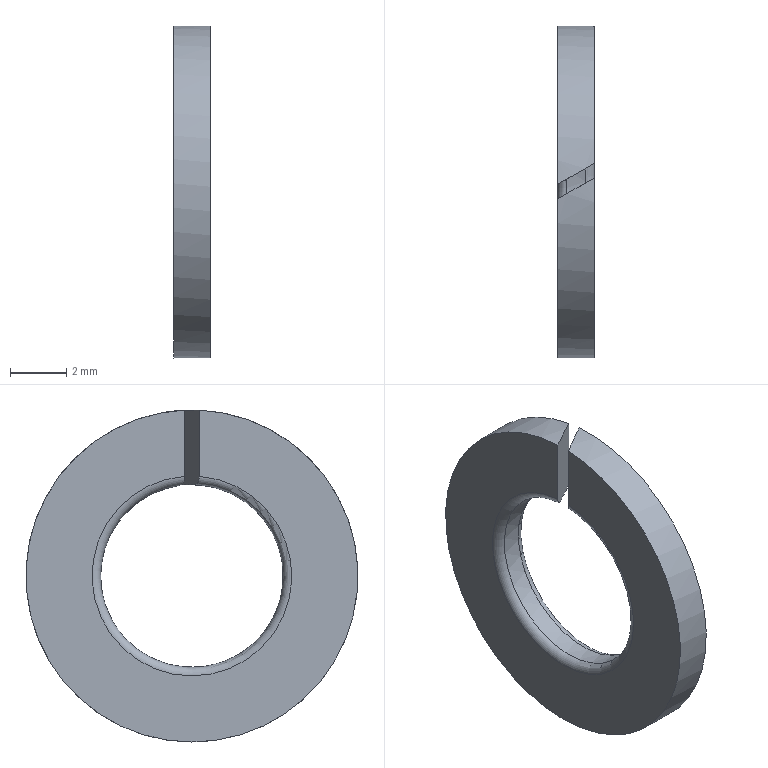Part | STEP file | DIN 128 - A6 | 1 solid | 8 faces | box 1.3 x 11.8 x 11.8 mm | volume 96.442 mm3 | plane 4 | cylinder 2 | torus 2 | commonest cylinder face diameters 6.5 x1 11.8 x1
STEP:
#1=CARTESIAN_POINT('',(0.,0.,0.));
#2=DIRECTION('',(0.,0.,1.));
#3=DIRECTION('',(1.,0.,0.));
#4=AXIS2_PLACEMENT_3D('',#1,#2,#3);
#5=CARTESIAN_POINT('',(1.3,1.011,3.403));
#6=VERTEX_POINT('',#5);
#7=CARTESIAN_POINT('',(1.,0.8374,3.14));
#8=VERTEX_POINT('',#7);
#9=CARTESIAN_POINT('',(1.3,1.011,3.403));
#10=CARTESIAN_POINT('',(1.3,1.011,3.366));
#11=CARTESIAN_POINT('',(1.292,1.006,3.323));
#12=CARTESIAN_POINT('',(1.265,0.9903,3.257));
#13=CARTESIAN_POINT('',(1.241,0.9768,3.224));
#14=CARTESIAN_POINT('',(1.191,0.9476,3.177));
#15=CARTESIAN_POINT('',(1.155,0.9267,3.157));
#16=CARTESIAN_POINT('',(1.085,0.8863,3.137));
#17=CARTESIAN_POINT('',(1.038,0.8595,3.134));
#18=CARTESIAN_POINT('',(1.,0.8374,3.14));
#19=B_SPLINE_CURVE_WITH_KNOTS('',3,(#9,#10,#11,#12,#13,#14,#15,#16,#17,#18),.UNSPECIFIED.,.F.,.F.,(4,2,2,2,4),(0.05089,0.06193,0.07271,0.08431,0.09772),.UNSPECIFIED.);
#20=CARTESIAN_POINT('',(0.,0.26,0.));
#21=DIRECTION('',(-0.5,0.866,0.));
#22=DIRECTION('',(0.,0.,1.));
#23=AXIS2_PLACEMENT_3D('',#20,#21,#22);
#24=PLANE('',#23);
#25=CARTESIAN_POINT('',(3.403,1.501));
#26=CARTESIAN_POINT('',(3.366,1.501));
#27=CARTESIAN_POINT('',(3.323,1.492));
#28=CARTESIAN_POINT('',(3.257,1.461));
#29=CARTESIAN_POINT('',(3.224,1.434));
#30=CARTESIAN_POINT('',(3.177,1.375));
#31=CARTESIAN_POINT('',(3.157,1.333));
#32=CARTESIAN_POINT('',(3.137,1.253));
#33=CARTESIAN_POINT('',(3.134,1.199));
#34=CARTESIAN_POINT('',(3.14,1.155));
#35=B_SPLINE_CURVE_WITH_KNOTS('',3,(#25,#26,#27,#28,#29,#30,#31,#32,#33,#34),.UNSPECIFIED.,.F.,.F.,(4,2,2,2,4),(0.05089,0.06193,0.07271,0.08431,0.09772),.UNSPECIFIED.);
#36=(GEOMETRIC_REPRESENTATION_CONTEXT(2)PARAMETRIC_REPRESENTATION_CONTEXT()REPRESENTATION_CONTEXT('',''));
#37=DEFINITIONAL_REPRESENTATION('',(#35),#36);
#38=PCURVE('',#24,#37);
#39=CARTESIAN_POINT('',(1.,0.,0.));
#40=DIRECTION('',(-1.,0.,0.));
#41=DIRECTION('',(0.,0.,1.));
#42=AXIS2_PLACEMENT_3D('',#39,#40,#41);
#43=TOROIDAL_SURFACE('',#42,3.55,0.3);
#44=CARTESIAN_POINT('',(0.2887,4.712));
#45=CARTESIAN_POINT('',(0.2892,4.69));
#46=CARTESIAN_POINT('',(0.2903,4.643));
#47=CARTESIAN_POINT('',(0.2918,4.568));
#48=CARTESIAN_POINT('',(0.293,4.492));
#49=CARTESIAN_POINT('',(0.2939,4.416));
#50=CARTESIAN_POINT('',(0.2945,4.343));
#51=CARTESIAN_POINT('',(0.2948,4.271));
#52=CARTESIAN_POINT('',(0.2947,4.195));
#53=CARTESIAN_POINT('',(0.2942,4.118));
#54=CARTESIAN_POINT('',(0.2935,4.041));
#55=CARTESIAN_POINT('',(0.2925,3.968));
#56=CARTESIAN_POINT('',(0.2911,3.899));
#57=CARTESIAN_POINT('',(0.2894,3.825));
#58=CARTESIAN_POINT('',(0.2874,3.751));
#59=CARTESIAN_POINT('',(0.2851,3.678));
#60=CARTESIAN_POINT('',(0.2826,3.607));
#61=CARTESIAN_POINT('',(0.2801,3.542));
#62=CARTESIAN_POINT('',(0.2773,3.475));
#63=CARTESIAN_POINT('',(0.2741,3.407));
#64=CARTESIAN_POINT('',(0.2708,3.338));
#65=CARTESIAN_POINT('',(0.2674,3.27));
#66=CARTESIAN_POINT('',(0.264,3.204));
#67=CARTESIAN_POINT('',(0.2617,3.162));
#68=CARTESIAN_POINT('',(0.2606,3.142));
#69=B_SPLINE_CURVE_WITH_KNOTS('',3,(#44,#45,#46,#47,#48,#49,#50,#51,#52,#53,#54,#55,#56,#57,#58,#59,#60,#61,#62,#63,#64,#65,#66,#67,#68),.UNSPECIFIED.,.F.,.F.,(4,1,1,1,1,1,1,1,1,1,1,1,1,1,1,1,1,1,1,1,1,1,4),(0.05089,0.05301,0.05514,0.05727,0.0594,0.06153,0.06366,0.06579,0.06792,0.07005,0.07217,0.0743,0.07643,0.07856,0.08069,0.08282,0.08495,0.08708,0.08921,0.09133,0.09346,0.09559,0.09772),.QUASI_UNIFORM_KNOTS.);
#70=(GEOMETRIC_REPRESENTATION_CONTEXT(2)PARAMETRIC_REPRESENTATION_CONTEXT()REPRESENTATION_CONTEXT('',''));
#71=DEFINITIONAL_REPRESENTATION('',(#69),#70);
#72=PCURVE('',#43,#71);
#73=SURFACE_CURVE('',#19,(#38,#72),.PCURVE_S1.);
#74=EDGE_CURVE('',#6,#8,#73,.T.);
#75=ORIENTED_EDGE('',*,*,#74,.F.);
#76=CARTESIAN_POINT('',(1.3,1.011,5.813));
#77=VERTEX_POINT('',#76);
#78=CARTESIAN_POINT('',(1.3,1.011,0.));
#79=DIRECTION('',(0.,0.,-1.));
#80=VECTOR('',#79,1.);
#81=LINE('',#78,#80);
#82=CARTESIAN_POINT('',(0.,1.501));
#83=DIRECTION('',(-1.,0.));
#84=VECTOR('',#83,1.);
#85=LINE('',#82,#84);
#86=(GEOMETRIC_REPRESENTATION_CONTEXT(2)PARAMETRIC_REPRESENTATION_CONTEXT()REPRESENTATION_CONTEXT('',''));
#87=DEFINITIONAL_REPRESENTATION('',(#85),#86);
#88=PCURVE('',#24,#87);
#89=CARTESIAN_POINT('',(1.3,0.,0.));
#90=DIRECTION('',(-1.,0.,0.));
#91=DIRECTION('',(0.,0.,1.));
#92=AXIS2_PLACEMENT_3D('',#89,#90,#91);
#93=PLANE('',#92);
#94=CARTESIAN_POINT('',(0.,1.011));
#95=DIRECTION('',(-1.,0.));
#96=VECTOR('',#95,1.);
#97=LINE('',#94,#96);
#98=(GEOMETRIC_REPRESENTATION_CONTEXT(2)PARAMETRIC_REPRESENTATION_CONTEXT()REPRESENTATION_CONTEXT('',''));
#99=DEFINITIONAL_REPRESENTATION('',(#97),#98);
#100=PCURVE('',#93,#99);
#101=SURFACE_CURVE('',#81,(#88,#100),.PCURVE_S1.);
#102=EDGE_CURVE('',#77,#6,#101,.T.);
#103=ORIENTED_EDGE('',*,*,#102,.F.);
#104=CARTESIAN_POINT('',(0.,0.26,5.894));
#105=VERTEX_POINT('',#104);
#106=CARTESIAN_POINT('',(-0.4503,0.,0.));
#107=DIRECTION('',(-0.5,0.866,0.));
#108=DIRECTION('',(-0.866,-0.5,0.));
#109=AXIS2_PLACEMENT_3D('',#106,#107,#108);
#110=ELLIPSE('',#109,11.8,5.9);
#111=CARTESIAN_POINT('',(0.,-0.52));
#112=DIRECTION('',(0.,-1.));
#113=AXIS2_PLACEMENT_2D('',#111,#112);
#114=ELLIPSE('',#113,11.8,5.9);
#115=(GEOMETRIC_REPRESENTATION_CONTEXT(2)PARAMETRIC_REPRESENTATION_CONTEXT()REPRESENTATION_CONTEXT('',''));
#116=DEFINITIONAL_REPRESENTATION('',(#114),#115);
#117=PCURVE('',#24,#116);
#118=CARTESIAN_POINT('',(0.,0.,0.));
#119=DIRECTION('',(1.,0.,0.));
#120=DIRECTION('',(0.,-1.,0.));
#121=AXIS2_PLACEMENT_3D('',#118,#119,#120);
#122=CYLINDRICAL_SURFACE('',#121,5.9);
#123=CARTESIAN_POINT('',(4.668,0.));
#124=CARTESIAN_POINT('',(4.54,1.3));
#125=B_SPLINE_CURVE_WITH_KNOTS('',1,(#123,#124),.UNSPECIFIED.,.F.,.F.,(2,2),(1.615,1.743),.PIECEWISE_BEZIER_KNOTS.);
#126=(GEOMETRIC_REPRESENTATION_CONTEXT(2)PARAMETRIC_REPRESENTATION_CONTEXT()REPRESENTATION_CONTEXT('',''));
#127=DEFINITIONAL_REPRESENTATION('',(#125),#126);
#128=PCURVE('',#122,#127);
#129=SURFACE_CURVE('',#110,(#117,#128),.PCURVE_S1.);
#130=EDGE_CURVE('',#105,#77,#129,.T.);
#131=ORIENTED_EDGE('',*,*,#130,.F.);
#132=CARTESIAN_POINT('',(0.,0.26,3.54));
#133=VERTEX_POINT('',#132);
#134=CARTESIAN_POINT('',(0.,0.26,0.));
#135=DIRECTION('',(0.,0.,1.));
#136=VECTOR('',#135,1.);
#137=LINE('',#134,#136);
#138=CARTESIAN_POINT('',(0.,0.));
#139=DIRECTION('',(1.,0.));
#140=VECTOR('',#139,1.);
#141=LINE('',#138,#140);
#142=(GEOMETRIC_REPRESENTATION_CONTEXT(2)PARAMETRIC_REPRESENTATION_CONTEXT()REPRESENTATION_CONTEXT('',''));
#143=DEFINITIONAL_REPRESENTATION('',(#141),#142);
#144=PCURVE('',#24,#143);
#145=CARTESIAN_POINT('',(0.,0.,0.));
#146=DIRECTION('',(-1.,0.,0.));
#147=DIRECTION('',(0.,0.,1.));
#148=AXIS2_PLACEMENT_3D('',#145,#146,#147);
#149=PLANE('',#148);
#150=CARTESIAN_POINT('',(0.,0.26));
#151=DIRECTION('',(1.,0.));
#152=VECTOR('',#151,1.);
#153=LINE('',#150,#152);
#154=(GEOMETRIC_REPRESENTATION_CONTEXT(2)PARAMETRIC_REPRESENTATION_CONTEXT()REPRESENTATION_CONTEXT('',''));
#155=DEFINITIONAL_REPRESENTATION('',(#153),#154);
#156=PCURVE('',#149,#155);
#157=SURFACE_CURVE('',#137,(#144,#156),.PCURVE_S1.);
#158=EDGE_CURVE('',#133,#105,#157,.T.);
#159=ORIENTED_EDGE('',*,*,#158,.F.);
#160=CARTESIAN_POINT('',(0.3,0.4332,3.221));
#161=VERTEX_POINT('',#160);
#162=CARTESIAN_POINT('',(0.3,0.4332,3.221));
#163=CARTESIAN_POINT('',(0.2609,0.4106,3.224));
#164=CARTESIAN_POINT('',(0.2152,0.3843,3.237));
#165=CARTESIAN_POINT('',(0.1453,0.3439,3.272));
#166=CARTESIAN_POINT('',(0.108,0.3224,3.301));
#167=CARTESIAN_POINT('',(0.05715,0.293,3.358));
#168=CARTESIAN_POINT('',(0.03356,0.2794,3.396));
#169=CARTESIAN_POINT('',(0.007847,0.2645,3.464));
#170=CARTESIAN_POINT('',(0.,0.26,3.505));
#171=CARTESIAN_POINT('',(0.,0.26,3.54));
#172=B_SPLINE_CURVE_WITH_KNOTS('',3,(#162,#163,#164,#165,#166,#167,#168,#169,#170,#171),.UNSPECIFIED.,.F.,.F.,(4,2,2,2,4),(0.09642,0.11,0.1229,0.1346,0.1452),.UNSPECIFIED.);
#173=CARTESIAN_POINT('',(3.221,0.3464));
#174=CARTESIAN_POINT('',(3.224,0.3013));
#175=CARTESIAN_POINT('',(3.237,0.2485));
#176=CARTESIAN_POINT('',(3.272,0.1678));
#177=CARTESIAN_POINT('',(3.301,0.1247));
#178=CARTESIAN_POINT('',(3.358,0.066));
#179=CARTESIAN_POINT('',(3.396,0.03875));
#180=CARTESIAN_POINT('',(3.464,0.009061));
#181=CARTESIAN_POINT('',(3.505,0.));
#182=CARTESIAN_POINT('',(3.54,0.));
#183=B_SPLINE_CURVE_WITH_KNOTS('',3,(#173,#174,#175,#176,#177,#178,#179,#180,#181,#182),.UNSPECIFIED.,.F.,.F.,(4,2,2,2,4),(0.09642,0.11,0.1229,0.1346,0.1452),.UNSPECIFIED.);
#184=(GEOMETRIC_REPRESENTATION_CONTEXT(2)PARAMETRIC_REPRESENTATION_CONTEXT()REPRESENTATION_CONTEXT('',''));
#185=DEFINITIONAL_REPRESENTATION('',(#183),#184);
#186=PCURVE('',#24,#185);
#187=CARTESIAN_POINT('',(0.3,0.,0.));
#188=DIRECTION('',(1.,0.,0.));
#189=DIRECTION('',(0.,0.,-1.));
#190=AXIS2_PLACEMENT_3D('',#187,#188,#189);
#191=TOROIDAL_SURFACE('',#190,3.55,0.3);
#192=CARTESIAN_POINT('',(9.291,3.142));
#193=CARTESIAN_POINT('',(9.292,3.163));
#194=CARTESIAN_POINT('',(9.295,3.207));
#195=CARTESIAN_POINT('',(9.298,3.275));
#196=CARTESIAN_POINT('',(9.302,3.344));
#197=CARTESIAN_POINT('',(9.306,3.413));
#198=CARTESIAN_POINT('',(9.31,3.482));
#199=CARTESIAN_POINT('',(9.313,3.547));
#200=CARTESIAN_POINT('',(9.317,3.612));
#201=CARTESIAN_POINT('',(9.32,3.681));
#202=CARTESIAN_POINT('',(9.324,3.752));
#203=CARTESIAN_POINT('',(9.327,3.824));
#204=CARTESIAN_POINT('',(9.33,3.895));
#205=CARTESIAN_POINT('',(9.333,3.962));
#206=CARTESIAN_POINT('',(9.336,4.031));
#207=CARTESIAN_POINT('',(9.339,4.105));
#208=CARTESIAN_POINT('',(9.341,4.18));
#209=CARTESIAN_POINT('',(9.343,4.256));
#210=CARTESIAN_POINT('',(9.345,4.329));
#211=CARTESIAN_POINT('',(9.347,4.401));
#212=CARTESIAN_POINT('',(9.349,4.479));
#213=CARTESIAN_POINT('',(9.35,4.558));
#214=CARTESIAN_POINT('',(9.351,4.637));
#215=CARTESIAN_POINT('',(9.351,4.688));
#216=CARTESIAN_POINT('',(9.351,4.712));
#217=B_SPLINE_CURVE_WITH_KNOTS('',3,(#192,#193,#194,#195,#196,#197,#198,#199,#200,#201,#202,#203,#204,#205,#206,#207,#208,#209,#210,#211,#212,#213,#214,#215,#216),.UNSPECIFIED.,.F.,.F.,(4,1,1,1,1,1,1,1,1,1,1,1,1,1,1,1,1,1,1,1,1,1,4),(0.09642,0.09863,0.1008,0.1031,0.1053,0.1075,0.1097,0.1119,0.1141,0.1164,0.1186,0.1208,0.123,0.1252,0.1274,0.1296,0.1319,0.1341,0.1363,0.1385,0.1407,0.1429,0.1452),.QUASI_UNIFORM_KNOTS.);
#218=(GEOMETRIC_REPRESENTATION_CONTEXT(2)PARAMETRIC_REPRESENTATION_CONTEXT()REPRESENTATION_CONTEXT('',''));
#219=DEFINITIONAL_REPRESENTATION('',(#217),#218);
#220=PCURVE('',#191,#219);
#221=SURFACE_CURVE('',#172,(#186,#220),.PCURVE_S1.);
#222=EDGE_CURVE('',#161,#133,#221,.T.);
#223=ORIENTED_EDGE('',*,*,#222,.F.);
#224=CARTESIAN_POINT('',(-0.4503,0.,0.));
#225=DIRECTION('',(0.5,-0.866,0.));
#226=DIRECTION('',(-0.866,-0.5,0.));
#227=AXIS2_PLACEMENT_3D('',#224,#225,#226);
#228=ELLIPSE('',#227,6.5,3.25);
#229=CARTESIAN_POINT('',(0.,-7.02));
#230=CARTESIAN_POINT('',(-5.629,-7.02));
#231=CARTESIAN_POINT('',(-2.815,2.73));
#232=CARTESIAN_POINT('',(0.,12.48));
#233=CARTESIAN_POINT('',(2.815,2.73));
#234=CARTESIAN_POINT('',(5.629,-7.02));
#235=CARTESIAN_POINT('',(0.,-7.02));
#236=(BOUNDED_CURVE()B_SPLINE_CURVE(2,(#229,#230,#231,#232,#233,#234,#235),.UNSPECIFIED.,.T.,.F.)B_SPLINE_CURVE_WITH_KNOTS((1,2,2,2,2,1),(-2.094,0.,2.094,4.189,6.283,8.378),.UNSPECIFIED.)CURVE()GEOMETRIC_REPRESENTATION_ITEM()RATIONAL_B_SPLINE_CURVE((1.,0.5,1.,0.5,1.,0.5,1.))REPRESENTATION_ITEM(''));
#237=(GEOMETRIC_REPRESENTATION_CONTEXT(2)PARAMETRIC_REPRESENTATION_CONTEXT()REPRESENTATION_CONTEXT('',''));
#238=DEFINITIONAL_REPRESENTATION('',(#236),#237);
#239=PCURVE('',#24,#238);
#240=CARTESIAN_POINT('',(0.,0.,0.));
#241=DIRECTION('',(1.,0.,0.));
#242=DIRECTION('',(0.,-1.,0.));
#243=AXIS2_PLACEMENT_3D('',#240,#241,#242);
#244=CYLINDRICAL_SURFACE('',#243,3.25);
#245=CARTESIAN_POINT('',(4.452,1.));
#246=CARTESIAN_POINT('',(4.579,0.3));
#247=B_SPLINE_CURVE_WITH_KNOTS('',1,(#245,#246),.UNSPECIFIED.,.F.,.F.,(2,2),(4.452,4.579),.PIECEWISE_BEZIER_KNOTS.);
#248=(GEOMETRIC_REPRESENTATION_CONTEXT(2)PARAMETRIC_REPRESENTATION_CONTEXT()REPRESENTATION_CONTEXT('',''));
#249=DEFINITIONAL_REPRESENTATION('',(#247),#248);
#250=PCURVE('',#244,#249);
#251=SURFACE_CURVE('',#228,(#239,#250),.PCURVE_S1.);
#252=EDGE_CURVE('',#8,#161,#251,.T.);
#253=ORIENTED_EDGE('',*,*,#252,.F.);
#254=EDGE_LOOP('',(#75,#103,#131,#159,#223,#253));
#255=FACE_BOUND('',#254,.T.);
#256=ADVANCED_FACE('',(#255),#24,.F.);
#257=CARTESIAN_POINT('',(1.,0.3174,3.234));
#258=VERTEX_POINT('',#257);
#259=CARTESIAN_POINT('',(1.3,0.4906,3.516));
#260=VERTEX_POINT('',#259);
#261=CARTESIAN_POINT('',(1.,0.3174,3.234));
#262=CARTESIAN_POINT('',(1.039,0.3398,3.232));
#263=CARTESIAN_POINT('',(1.085,0.3665,3.239));
#264=CARTESIAN_POINT('',(1.155,0.4069,3.265));
#265=CARTESIAN_POINT('',(1.192,0.4281,3.288));
#266=CARTESIAN_POINT('',(1.242,0.4573,3.339));
#267=CARTESIAN_POINT('',(1.266,0.4708,3.373));
#268=CARTESIAN_POINT('',(1.292,0.486,3.439));
#269=CARTESIAN_POINT('',(1.3,0.4906,3.48));
#270=CARTESIAN_POINT('',(1.3,0.4906,3.516));
#271=B_SPLINE_CURVE_WITH_KNOTS('',3,(#261,#262,#263,#264,#265,#266,#267,#268,#269,#270),.UNSPECIFIED.,.F.,.F.,(4,2,2,2,4),(0.09598,0.1094,0.1215,0.1325,0.1432),.UNSPECIFIED.);
#272=CARTESIAN_POINT('',(1.3,0.4906,0.));
#273=DIRECTION('',(0.5,-0.866,0.));
#274=DIRECTION('',(0.,0.,-1.));
#275=AXIS2_PLACEMENT_3D('',#272,#273,#274);
#276=PLANE('',#275);
#277=CARTESIAN_POINT('',(-3.234,-0.3464));
#278=CARTESIAN_POINT('',(-3.232,-0.3016));
#279=CARTESIAN_POINT('',(-3.239,-0.2481));
#280=CARTESIAN_POINT('',(-3.265,-0.1673));
#281=CARTESIAN_POINT('',(-3.288,-0.1249));
#282=CARTESIAN_POINT('',(-3.339,-0.06651));
#283=CARTESIAN_POINT('',(-3.373,-0.0395));
#284=CARTESIAN_POINT('',(-3.439,-0.009098));
#285=CARTESIAN_POINT('',(-3.48,0.));
#286=CARTESIAN_POINT('',(-3.516,0.));
#287=B_SPLINE_CURVE_WITH_KNOTS('',3,(#277,#278,#279,#280,#281,#282,#283,#284,#285,#286),.UNSPECIFIED.,.F.,.F.,(4,2,2,2,4),(0.09598,0.1094,0.1215,0.1325,0.1432),.UNSPECIFIED.);
#288=(GEOMETRIC_REPRESENTATION_CONTEXT(2)PARAMETRIC_REPRESENTATION_CONTEXT()REPRESENTATION_CONTEXT('',''));
#289=DEFINITIONAL_REPRESENTATION('',(#287),#288);
#290=PCURVE('',#276,#289);
#291=CARTESIAN_POINT('',(6.381,3.142));
#292=CARTESIAN_POINT('',(6.382,3.162));
#293=CARTESIAN_POINT('',(6.384,3.205));
#294=CARTESIAN_POINT('',(6.388,3.271));
#295=CARTESIAN_POINT('',(6.391,3.339));
#296=CARTESIAN_POINT('',(6.395,3.408));
#297=CARTESIAN_POINT('',(6.398,3.477));
#298=CARTESIAN_POINT('',(6.401,3.543));
#299=CARTESIAN_POINT('',(6.404,3.607));
#300=CARTESIAN_POINT('',(6.407,3.677));
#301=CARTESIAN_POINT('',(6.409,3.749));
#302=CARTESIAN_POINT('',(6.412,3.822));
#303=CARTESIAN_POINT('',(6.414,3.894));
#304=CARTESIAN_POINT('',(6.416,3.963));
#305=CARTESIAN_POINT('',(6.418,4.034));
#306=CARTESIAN_POINT('',(6.42,4.109));
#307=CARTESIAN_POINT('',(6.421,4.186));
#308=CARTESIAN_POINT('',(6.422,4.262));
#309=CARTESIAN_POINT('',(6.423,4.335));
#310=CARTESIAN_POINT('',(6.423,4.407));
#311=CARTESIAN_POINT('',(6.423,4.485));
#312=CARTESIAN_POINT('',(6.423,4.563));
#313=CARTESIAN_POINT('',(6.423,4.64));
#314=CARTESIAN_POINT('',(6.422,4.689));
#315=CARTESIAN_POINT('',(6.422,4.712));
#316=B_SPLINE_CURVE_WITH_KNOTS('',3,(#291,#292,#293,#294,#295,#296,#297,#298,#299,#300,#301,#302,#303,#304,#305,#306,#307,#308,#309,#310,#311,#312,#313,#314,#315),.UNSPECIFIED.,.F.,.F.,(4,1,1,1,1,1,1,1,1,1,1,1,1,1,1,1,1,1,1,1,1,1,4),(0.09598,0.09812,0.1003,0.1024,0.1046,0.1067,0.1088,0.111,0.1131,0.1153,0.1174,0.1196,0.1217,0.1239,0.126,0.1282,0.1303,0.1324,0.1346,0.1367,0.1389,0.141,0.1432),.QUASI_UNIFORM_KNOTS.);
#317=(GEOMETRIC_REPRESENTATION_CONTEXT(2)PARAMETRIC_REPRESENTATION_CONTEXT()REPRESENTATION_CONTEXT('',''));
#318=DEFINITIONAL_REPRESENTATION('',(#316),#317);
#319=PCURVE('',#43,#318);
#320=SURFACE_CURVE('',#271,(#290,#319),.PCURVE_S1.);
#321=EDGE_CURVE('',#258,#260,#320,.T.);
#322=ORIENTED_EDGE('',*,*,#321,.F.);
#323=CARTESIAN_POINT('',(0.3,-0.08679,3.249));
#324=VERTEX_POINT('',#323);
#325=CARTESIAN_POINT('',(0.4503,0.,0.));
#326=DIRECTION('',(-0.5,0.866,0.));
#327=DIRECTION('',(-0.866,-0.5,0.));
#328=AXIS2_PLACEMENT_3D('',#325,#326,#327);
#329=ELLIPSE('',#328,6.5,3.25);
#330=CARTESIAN_POINT('',(0.,-7.481));
#331=CARTESIAN_POINT('',(-5.629,-7.481));
#332=CARTESIAN_POINT('',(-2.815,2.269));
#333=CARTESIAN_POINT('',(0.,12.019));
#334=CARTESIAN_POINT('',(2.815,2.269));
#335=CARTESIAN_POINT('',(5.629,-7.481));
#336=CARTESIAN_POINT('',(0.,-7.481));
#337=(BOUNDED_CURVE()B_SPLINE_CURVE(2,(#330,#331,#332,#333,#334,#335,#336),.UNSPECIFIED.,.T.,.F.)B_SPLINE_CURVE_WITH_KNOTS((1,2,2,2,2,1),(-2.094,0.,2.094,4.189,6.283,8.378),.UNSPECIFIED.)CURVE()GEOMETRIC_REPRESENTATION_ITEM()RATIONAL_B_SPLINE_CURVE((1.,0.5,1.,0.5,1.,0.5,1.))REPRESENTATION_ITEM(''));
#338=(GEOMETRIC_REPRESENTATION_CONTEXT(2)PARAMETRIC_REPRESENTATION_CONTEXT()REPRESENTATION_CONTEXT('',''));
#339=DEFINITIONAL_REPRESENTATION('',(#337),#338);
#340=PCURVE('',#276,#339);
#341=CARTESIAN_POINT('',(-1.544,0.3));
#342=CARTESIAN_POINT('',(-1.669,1.));
#343=B_SPLINE_CURVE_WITH_KNOTS('',1,(#341,#342),.UNSPECIFIED.,.F.,.F.,(2,2),(1.544,1.669),.PIECEWISE_BEZIER_KNOTS.);
#344=(GEOMETRIC_REPRESENTATION_CONTEXT(2)PARAMETRIC_REPRESENTATION_CONTEXT()REPRESENTATION_CONTEXT('',''));
#345=DEFINITIONAL_REPRESENTATION('',(#343),#344);
#346=PCURVE('',#244,#345);
#347=SURFACE_CURVE('',#329,(#340,#346),.PCURVE_S1.);
#348=EDGE_CURVE('',#324,#258,#347,.T.);
#349=ORIENTED_EDGE('',*,*,#348,.F.);
#350=CARTESIAN_POINT('',(0.,-0.26,3.54));
#351=VERTEX_POINT('',#350);
#352=CARTESIAN_POINT('',(0.,-0.26,3.54));
#353=CARTESIAN_POINT('',(0.,-0.26,3.505));
#354=CARTESIAN_POINT('',(0.007853,-0.2555,3.464));
#355=CARTESIAN_POINT('',(0.03393,-0.2404,3.398));
#356=CARTESIAN_POINT('',(0.05736,-0.2269,3.362));
#357=CARTESIAN_POINT('',(0.108,-0.1977,3.31));
#358=CARTESIAN_POINT('',(0.1449,-0.1763,3.286));
#359=CARTESIAN_POINT('',(0.2149,-0.1359,3.257));
#360=CARTESIAN_POINT('',(0.2611,-0.1093,3.248));
#361=CARTESIAN_POINT('',(0.3,-0.08679,3.249));
#362=B_SPLINE_CURVE_WITH_KNOTS('',3,(#352,#353,#354,#355,#356,#357,#358,#359,#360,#361),.UNSPECIFIED.,.F.,.F.,(4,2,2,2,4),(0.04839,0.05895,0.07013,0.08242,0.09591),.UNSPECIFIED.);
#363=CARTESIAN_POINT('',(-3.54,-1.501));
#364=CARTESIAN_POINT('',(-3.505,-1.501));
#365=CARTESIAN_POINT('',(-3.464,-1.492));
#366=CARTESIAN_POINT('',(-3.398,-1.462));
#367=CARTESIAN_POINT('',(-3.362,-1.435));
#368=CARTESIAN_POINT('',(-3.31,-1.376));
#369=CARTESIAN_POINT('',(-3.286,-1.334));
#370=CARTESIAN_POINT('',(-3.257,-1.253));
#371=CARTESIAN_POINT('',(-3.248,-1.2));
#372=CARTESIAN_POINT('',(-3.249,-1.155));
#373=B_SPLINE_CURVE_WITH_KNOTS('',3,(#363,#364,#365,#366,#367,#368,#369,#370,#371,#372),.UNSPECIFIED.,.F.,.F.,(4,2,2,2,4),(0.04839,0.05895,0.07013,0.08242,0.09591),.UNSPECIFIED.);
#374=(GEOMETRIC_REPRESENTATION_CONTEXT(2)PARAMETRIC_REPRESENTATION_CONTEXT()REPRESENTATION_CONTEXT('',''));
#375=DEFINITIONAL_REPRESENTATION('',(#373),#374);
#376=PCURVE('',#276,#375);
#377=CARTESIAN_POINT('',(3.215,4.712));
#378=CARTESIAN_POINT('',(3.215,4.688));
#379=CARTESIAN_POINT('',(3.215,4.639));
#380=CARTESIAN_POINT('',(3.215,4.561));
#381=CARTESIAN_POINT('',(3.215,4.482));
#382=CARTESIAN_POINT('',(3.214,4.405));
#383=CARTESIAN_POINT('',(3.214,4.333));
#384=CARTESIAN_POINT('',(3.213,4.259));
#385=CARTESIAN_POINT('',(3.211,4.183));
#386=CARTESIAN_POINT('',(3.209,4.107));
#387=CARTESIAN_POINT('',(3.208,4.032));
#388=CARTESIAN_POINT('',(3.205,3.962));
#389=CARTESIAN_POINT('',(3.203,3.893));
#390=CARTESIAN_POINT('',(3.201,3.821));
#391=CARTESIAN_POINT('',(3.198,3.749));
#392=CARTESIAN_POINT('',(3.195,3.678));
#393=CARTESIAN_POINT('',(3.192,3.608));
#394=CARTESIAN_POINT('',(3.189,3.544));
#395=CARTESIAN_POINT('',(3.186,3.478));
#396=CARTESIAN_POINT('',(3.182,3.41));
#397=CARTESIAN_POINT('',(3.179,3.341));
#398=CARTESIAN_POINT('',(3.175,3.272));
#399=CARTESIAN_POINT('',(3.172,3.205));
#400=CARTESIAN_POINT('',(3.169,3.162));
#401=CARTESIAN_POINT('',(3.168,3.142));
#402=B_SPLINE_CURVE_WITH_KNOTS('',3,(#377,#378,#379,#380,#381,#382,#383,#384,#385,#386,#387,#388,#389,#390,#391,#392,#393,#394,#395,#396,#397,#398,#399,#400,#401),.UNSPECIFIED.,.F.,.F.,(4,1,1,1,1,1,1,1,1,1,1,1,1,1,1,1,1,1,1,1,1,1,4),(0.04839,0.05055,0.05271,0.05487,0.05703,0.05919,0.06135,0.06351,0.06567,0.06783,0.06999,0.07215,0.07431,0.07647,0.07863,0.08079,0.08295,0.08511,0.08727,0.08943,0.09159,0.09375,0.09591),.QUASI_UNIFORM_KNOTS.);
#403=(GEOMETRIC_REPRESENTATION_CONTEXT(2)PARAMETRIC_REPRESENTATION_CONTEXT()REPRESENTATION_CONTEXT('',''));
#404=DEFINITIONAL_REPRESENTATION('',(#402),#403);
#405=PCURVE('',#191,#404);
#406=SURFACE_CURVE('',#362,(#376,#405),.PCURVE_S1.);
#407=EDGE_CURVE('',#351,#324,#406,.T.);
#408=ORIENTED_EDGE('',*,*,#407,.F.);
#409=CARTESIAN_POINT('',(0.,-0.26,5.894));
#410=VERTEX_POINT('',#409);
#411=CARTESIAN_POINT('',(0.,-0.26,0.));
#412=DIRECTION('',(0.,0.,-1.));
#413=VECTOR('',#412,1.);
#414=LINE('',#411,#413);
#415=CARTESIAN_POINT('',(0.,-1.501));
#416=DIRECTION('',(1.,0.));
#417=VECTOR('',#416,1.);
#418=LINE('',#415,#417);
#419=(GEOMETRIC_REPRESENTATION_CONTEXT(2)PARAMETRIC_REPRESENTATION_CONTEXT()REPRESENTATION_CONTEXT('',''));
#420=DEFINITIONAL_REPRESENTATION('',(#418),#419);
#421=PCURVE('',#276,#420);
#422=CARTESIAN_POINT('',(0.,-0.26));
#423=DIRECTION('',(-1.,0.));
#424=VECTOR('',#423,1.);
#425=LINE('',#422,#424);
#426=(GEOMETRIC_REPRESENTATION_CONTEXT(2)PARAMETRIC_REPRESENTATION_CONTEXT()REPRESENTATION_CONTEXT('',''));
#427=DEFINITIONAL_REPRESENTATION('',(#425),#426);
#428=PCURVE('',#149,#427);
#429=SURFACE_CURVE('',#414,(#421,#428),.PCURVE_S1.);
#430=EDGE_CURVE('',#410,#351,#429,.T.);
#431=ORIENTED_EDGE('',*,*,#430,.F.);
#432=CARTESIAN_POINT('',(1.3,0.4906,5.88));
#433=VERTEX_POINT('',#432);
#434=CARTESIAN_POINT('',(0.4503,0.,0.));
#435=DIRECTION('',(0.5,-0.866,0.));
#436=DIRECTION('',(-0.866,-0.5,0.));
#437=AXIS2_PLACEMENT_3D('',#434,#435,#436);
#438=ELLIPSE('',#437,11.8,5.9);
#439=CARTESIAN_POINT('',(0.,-0.9811));
#440=DIRECTION('',(0.,-1.));
#441=AXIS2_PLACEMENT_2D('',#439,#440);
#442=ELLIPSE('',#441,11.8,5.9);
#443=(GEOMETRIC_REPRESENTATION_CONTEXT(2)PARAMETRIC_REPRESENTATION_CONTEXT()REPRESENTATION_CONTEXT('',''));
#444=DEFINITIONAL_REPRESENTATION('',(#442),#443);
#445=PCURVE('',#276,#444);
#446=CARTESIAN_POINT('',(-1.654,1.3));
#447=CARTESIAN_POINT('',(-1.527,0.));
#448=B_SPLINE_CURVE_WITH_KNOTS('',1,(#446,#447),.UNSPECIFIED.,.F.,.F.,(2,2),(4.629,4.756),.PIECEWISE_BEZIER_KNOTS.);
#449=(GEOMETRIC_REPRESENTATION_CONTEXT(2)PARAMETRIC_REPRESENTATION_CONTEXT()REPRESENTATION_CONTEXT('',''));
#450=DEFINITIONAL_REPRESENTATION('',(#448),#449);
#451=PCURVE('',#122,#450);
#452=SURFACE_CURVE('',#438,(#445,#451),.PCURVE_S1.);
#453=EDGE_CURVE('',#433,#410,#452,.T.);
#454=ORIENTED_EDGE('',*,*,#453,.F.);
#455=CARTESIAN_POINT('',(1.3,0.4906,0.));
#456=DIRECTION('',(0.,0.,1.));
#457=VECTOR('',#456,1.);
#458=LINE('',#455,#457);
#459=CARTESIAN_POINT('',(0.,0.));
#460=DIRECTION('',(-1.,0.));
#461=VECTOR('',#460,1.);
#462=LINE('',#459,#461);
#463=(GEOMETRIC_REPRESENTATION_CONTEXT(2)PARAMETRIC_REPRESENTATION_CONTEXT()REPRESENTATION_CONTEXT('',''));
#464=DEFINITIONAL_REPRESENTATION('',(#462),#463);
#465=PCURVE('',#276,#464);
#466=CARTESIAN_POINT('',(0.,0.4906));
#467=DIRECTION('',(1.,0.));
#468=VECTOR('',#467,1.);
#469=LINE('',#466,#468);
#470=(GEOMETRIC_REPRESENTATION_CONTEXT(2)PARAMETRIC_REPRESENTATION_CONTEXT()REPRESENTATION_CONTEXT('',''));
#471=DEFINITIONAL_REPRESENTATION('',(#469),#470);
#472=PCURVE('',#93,#471);
#473=SURFACE_CURVE('',#458,(#465,#472),.PCURVE_S1.);
#474=EDGE_CURVE('',#260,#433,#473,.T.);
#475=ORIENTED_EDGE('',*,*,#474,.F.);
#476=EDGE_LOOP('',(#322,#349,#408,#431,#454,#475));
#477=FACE_BOUND('',#476,.T.);
#478=ADVANCED_FACE('',(#477),#276,.F.);
#479=CARTESIAN_POINT('',(1.,0.,0.));
#480=DIRECTION('',(-1.,0.,0.));
#481=DIRECTION('',(0.,-1.,0.));
#482=AXIS2_PLACEMENT_3D('',#479,#480,#481);
#483=CIRCLE('',#482,3.25);
#484=CARTESIAN_POINT('',(6.283,1.));
#485=DIRECTION('',(-1.,0.));
#486=VECTOR('',#485,1.);
#487=LINE('',#484,#486);
#488=(GEOMETRIC_REPRESENTATION_CONTEXT(2)PARAMETRIC_REPRESENTATION_CONTEXT()REPRESENTATION_CONTEXT('',''));
#489=DEFINITIONAL_REPRESENTATION('',(#487),#488);
#490=PCURVE('',#244,#489);
#491=CARTESIAN_POINT('',(-1.571,3.142));
#492=DIRECTION('',(1.,0.));
#493=VECTOR('',#492,1.);
#494=LINE('',#491,#493);
#495=(GEOMETRIC_REPRESENTATION_CONTEXT(2)PARAMETRIC_REPRESENTATION_CONTEXT()REPRESENTATION_CONTEXT('',''));
#496=DEFINITIONAL_REPRESENTATION('',(#494),#495);
#497=PCURVE('',#43,#496);
#498=SURFACE_CURVE('',#483,(#490,#497),.PCURVE_S1.);
#499=EDGE_CURVE('',#8,#258,#498,.T.);
#500=ORIENTED_EDGE('',*,*,#499,.T.);
#501=ORIENTED_EDGE('',*,*,#348,.F.);
#502=CARTESIAN_POINT('',(0.3,0.,0.));
#503=DIRECTION('',(1.,0.,0.));
#504=DIRECTION('',(0.,-1.,0.));
#505=AXIS2_PLACEMENT_3D('',#502,#503,#504);
#506=CIRCLE('',#505,3.25);
#507=CARTESIAN_POINT('',(-6.283,0.3));
#508=DIRECTION('',(1.,0.));
#509=VECTOR('',#508,1.);
#510=LINE('',#507,#509);
#511=(GEOMETRIC_REPRESENTATION_CONTEXT(2)PARAMETRIC_REPRESENTATION_CONTEXT()REPRESENTATION_CONTEXT('',''));
#512=DEFINITIONAL_REPRESENTATION('',(#510),#511);
#513=PCURVE('',#244,#512);
#514=CARTESIAN_POINT('',(-1.571,3.142));
#515=DIRECTION('',(1.,0.));
#516=VECTOR('',#515,1.);
#517=LINE('',#514,#516);
#518=(GEOMETRIC_REPRESENTATION_CONTEXT(2)PARAMETRIC_REPRESENTATION_CONTEXT()REPRESENTATION_CONTEXT('',''));
#519=DEFINITIONAL_REPRESENTATION('',(#517),#518);
#520=PCURVE('',#191,#519);
#521=SURFACE_CURVE('',#506,(#513,#520),.PCURVE_S1.);
#522=EDGE_CURVE('',#324,#161,#521,.T.);
#523=ORIENTED_EDGE('',*,*,#522,.T.);
#524=ORIENTED_EDGE('',*,*,#252,.F.);
#525=EDGE_LOOP('',(#500,#501,#523,#524));
#526=FACE_BOUND('',#525,.F.);
#527=ADVANCED_FACE('',(#526),#244,.F.);
#528=ORIENTED_EDGE('',*,*,#222,.T.);
#529=CARTESIAN_POINT('',(0.,0.,0.));
#530=DIRECTION('',(-1.,0.,0.));
#531=DIRECTION('',(0.,-1.,0.));
#532=AXIS2_PLACEMENT_3D('',#529,#530,#531);
#533=CIRCLE('',#532,3.55);
#534=CARTESIAN_POINT('',(10.996,4.712));
#535=DIRECTION('',(-1.,0.));
#536=VECTOR('',#535,1.);
#537=LINE('',#534,#536);
#538=(GEOMETRIC_REPRESENTATION_CONTEXT(2)PARAMETRIC_REPRESENTATION_CONTEXT()REPRESENTATION_CONTEXT('',''));
#539=DEFINITIONAL_REPRESENTATION('',(#537),#538);
#540=PCURVE('',#191,#539);
#541=CARTESIAN_POINT('',(0.,0.));
#542=DIRECTION('',(0.,-1.));
#543=AXIS2_PLACEMENT_2D('',#541,#542);
#544=CIRCLE('',#543,3.55);
#545=(GEOMETRIC_REPRESENTATION_CONTEXT(2)PARAMETRIC_REPRESENTATION_CONTEXT()REPRESENTATION_CONTEXT('',''));
#546=DEFINITIONAL_REPRESENTATION('',(#544),#545);
#547=PCURVE('',#149,#546);
#548=SURFACE_CURVE('',#533,(#540,#547),.PCURVE_S1.);
#549=EDGE_CURVE('',#133,#351,#548,.T.);
#550=ORIENTED_EDGE('',*,*,#549,.T.);
#551=ORIENTED_EDGE('',*,*,#407,.T.);
#552=ORIENTED_EDGE('',*,*,#522,.T.);
#553=EDGE_LOOP('',(#528,#550,#551,#552));
#554=FACE_BOUND('',#553,.T.);
#555=ADVANCED_FACE('',(#554),#191,.T.);
#556=ORIENTED_EDGE('',*,*,#158,.T.);
#557=CARTESIAN_POINT('',(0.,0.,0.));
#558=DIRECTION('',(-1.,0.,0.));
#559=DIRECTION('',(0.,-1.,0.));
#560=AXIS2_PLACEMENT_3D('',#557,#558,#559);
#561=CIRCLE('',#560,5.9);
#562=CARTESIAN_POINT('',(0.,0.));
#563=DIRECTION('',(0.,-1.));
#564=AXIS2_PLACEMENT_2D('',#562,#563);
#565=CIRCLE('',#564,5.9);
#566=(GEOMETRIC_REPRESENTATION_CONTEXT(2)PARAMETRIC_REPRESENTATION_CONTEXT()REPRESENTATION_CONTEXT('',''));
#567=DEFINITIONAL_REPRESENTATION('',(#565),#566);
#568=PCURVE('',#149,#567);
#569=CARTESIAN_POINT('',(6.283,0.));
#570=DIRECTION('',(-1.,0.));
#571=VECTOR('',#570,1.);
#572=LINE('',#569,#571);
#573=(GEOMETRIC_REPRESENTATION_CONTEXT(2)PARAMETRIC_REPRESENTATION_CONTEXT()REPRESENTATION_CONTEXT('',''));
#574=DEFINITIONAL_REPRESENTATION('',(#572),#573);
#575=PCURVE('',#122,#574);
#576=SURFACE_CURVE('',#561,(#568,#575),.PCURVE_S1.);
#577=EDGE_CURVE('',#105,#410,#576,.T.);
#578=ORIENTED_EDGE('',*,*,#577,.T.);
#579=ORIENTED_EDGE('',*,*,#430,.T.);
#580=ORIENTED_EDGE('',*,*,#549,.F.);
#581=EDGE_LOOP('',(#556,#578,#579,#580));
#582=FACE_BOUND('',#581,.T.);
#583=ADVANCED_FACE('',(#582),#149,.T.);
#584=ORIENTED_EDGE('',*,*,#74,.T.);
#585=ORIENTED_EDGE('',*,*,#499,.T.);
#586=ORIENTED_EDGE('',*,*,#321,.T.);
#587=CARTESIAN_POINT('',(1.3,0.,0.));
#588=DIRECTION('',(1.,0.,0.));
#589=DIRECTION('',(0.,-1.,0.));
#590=AXIS2_PLACEMENT_3D('',#587,#588,#589);
#591=CIRCLE('',#590,3.55);
#592=CARTESIAN_POINT('',(10.996,4.712));
#593=DIRECTION('',(-1.,0.));
#594=VECTOR('',#593,1.);
#595=LINE('',#592,#594);
#596=(GEOMETRIC_REPRESENTATION_CONTEXT(2)PARAMETRIC_REPRESENTATION_CONTEXT()REPRESENTATION_CONTEXT('',''));
#597=DEFINITIONAL_REPRESENTATION('',(#595),#596);
#598=PCURVE('',#43,#597);
#599=CARTESIAN_POINT('',(0.,-3.55));
#600=CARTESIAN_POINT('',(-6.149,-3.55));
#601=CARTESIAN_POINT('',(-3.074,1.775));
#602=CARTESIAN_POINT('',(0.,7.1));
#603=CARTESIAN_POINT('',(3.074,1.775));
#604=CARTESIAN_POINT('',(6.149,-3.55));
#605=CARTESIAN_POINT('',(0.,-3.55));
#606=(BOUNDED_CURVE()B_SPLINE_CURVE(2,(#599,#600,#601,#602,#603,#604,#605),.UNSPECIFIED.,.T.,.F.)B_SPLINE_CURVE_WITH_KNOTS((1,2,2,2,2,1),(-2.094,0.,2.094,4.189,6.283,8.378),.UNSPECIFIED.)CURVE()GEOMETRIC_REPRESENTATION_ITEM()RATIONAL_B_SPLINE_CURVE((1.,0.5,1.,0.5,1.,0.5,1.))REPRESENTATION_ITEM(''));
#607=(GEOMETRIC_REPRESENTATION_CONTEXT(2)PARAMETRIC_REPRESENTATION_CONTEXT()REPRESENTATION_CONTEXT('',''));
#608=DEFINITIONAL_REPRESENTATION('',(#606),#607);
#609=PCURVE('',#93,#608);
#610=SURFACE_CURVE('',#591,(#598,#609),.PCURVE_S1.);
#611=EDGE_CURVE('',#260,#6,#610,.T.);
#612=ORIENTED_EDGE('',*,*,#611,.T.);
#613=EDGE_LOOP('',(#584,#585,#586,#612));
#614=FACE_BOUND('',#613,.T.);
#615=ADVANCED_FACE('',(#614),#43,.T.);
#616=ORIENTED_EDGE('',*,*,#102,.T.);
#617=ORIENTED_EDGE('',*,*,#611,.F.);
#618=ORIENTED_EDGE('',*,*,#474,.T.);
#619=CARTESIAN_POINT('',(1.3,0.,0.));
#620=DIRECTION('',(-1.,0.,0.));
#621=DIRECTION('',(0.,-1.,0.));
#622=AXIS2_PLACEMENT_3D('',#619,#620,#621);
#623=CIRCLE('',#622,5.9);
#624=CARTESIAN_POINT('',(0.,0.));
#625=DIRECTION('',(0.,-1.));
#626=AXIS2_PLACEMENT_2D('',#624,#625);
#627=CIRCLE('',#626,5.9);
#628=(GEOMETRIC_REPRESENTATION_CONTEXT(2)PARAMETRIC_REPRESENTATION_CONTEXT()REPRESENTATION_CONTEXT('',''));
#629=DEFINITIONAL_REPRESENTATION('',(#627),#628);
#630=PCURVE('',#93,#629);
#631=CARTESIAN_POINT('',(6.283,1.3));
#632=DIRECTION('',(-1.,0.));
#633=VECTOR('',#632,1.);
#634=LINE('',#631,#633);
#635=(GEOMETRIC_REPRESENTATION_CONTEXT(2)PARAMETRIC_REPRESENTATION_CONTEXT()REPRESENTATION_CONTEXT('',''));
#636=DEFINITIONAL_REPRESENTATION('',(#634),#635);
#637=PCURVE('',#122,#636);
#638=SURFACE_CURVE('',#623,(#630,#637),.PCURVE_S1.);
#639=EDGE_CURVE('',#77,#433,#638,.T.);
#640=ORIENTED_EDGE('',*,*,#639,.F.);
#641=EDGE_LOOP('',(#616,#617,#618,#640));
#642=FACE_BOUND('',#641,.T.);
#643=ADVANCED_FACE('',(#642),#93,.F.);
#644=ORIENTED_EDGE('',*,*,#130,.T.);
#645=ORIENTED_EDGE('',*,*,#639,.T.);
#646=ORIENTED_EDGE('',*,*,#453,.T.);
#647=ORIENTED_EDGE('',*,*,#577,.F.);
#648=EDGE_LOOP('',(#644,#645,#646,#647));
#649=FACE_BOUND('',#648,.T.);
#650=ADVANCED_FACE('',(#649),#122,.T.);
#651=CLOSED_SHELL('',(#256,#478,#527,#555,#583,#615,#643,#650));
#652=MANIFOLD_SOLID_BREP('',#651);
#653=(LENGTH_UNIT()NAMED_UNIT(*)SI_UNIT(.MILLI.,.METRE.));
#654=UNCERTAINTY_MEASURE_WITH_UNIT(LENGTH_MEASURE(0.001),#653,'','');
#655=(NAMED_UNIT(*)PLANE_ANGLE_UNIT()SI_UNIT($,.RADIAN.));
#656=(NAMED_UNIT(*)SI_UNIT($,.STERADIAN.)SOLID_ANGLE_UNIT());
#657=(GEOMETRIC_REPRESENTATION_CONTEXT(3)GLOBAL_UNCERTAINTY_ASSIGNED_CONTEXT((#654))GLOBAL_UNIT_ASSIGNED_CONTEXT((#653,#655,#656))REPRESENTATION_CONTEXT('',''));
#658=ADVANCED_BREP_SHAPE_REPRESENTATION('',(#4,#652),#657);